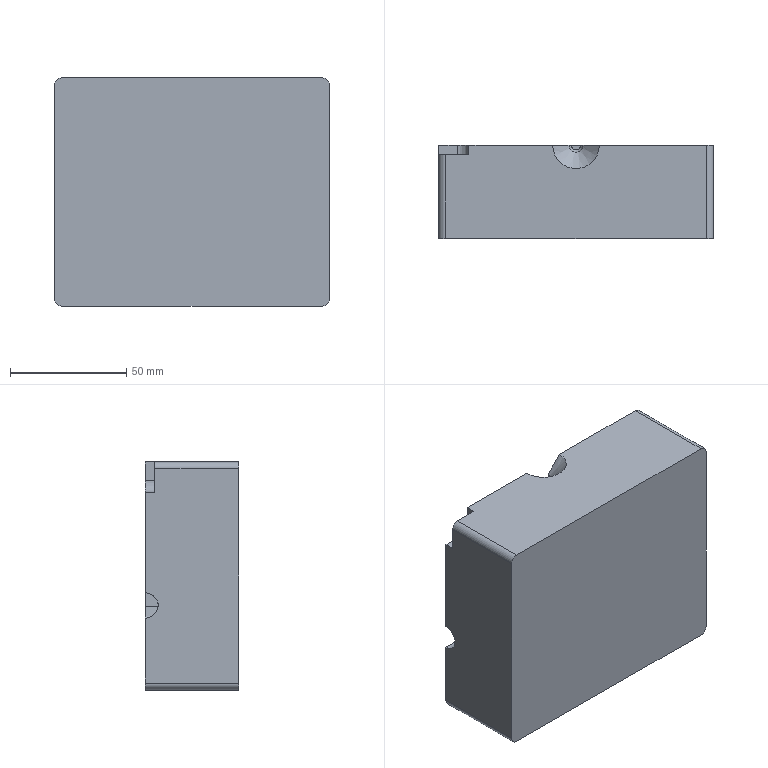NC program | NX | posted with a generic post | part box 118 x 40 x 98 mm
Lines 34771 to 36173 of 39656:
(ZLEVEL_PROFILE , TOOL : D8R1)
N69516 M6
N69518 G54
N69520 G17 G0 G90 X14.157 Y-3.614 S0 M3
N69522 G43 Z30. H0
N69524 Z3.
N69526 G94 G1 Z-5. F250.
N69528 G2 X13.635 Y-1.241 R6.575
N69530 G1 X13.195 Y13.066
N69532 G3 X-13.195 Y13.066 R13.201
N69534 G1 X-13.635 Y-1.241
N69536 G2 X-14.157 Y-3.614 R6.575
N69538 G1 Z-8.446
N69540 G3 X-13.635 Y-1.241 R6.575
N69542 G1 X-13.195 Y13.066
N69544 G2 X13.195 Y13.066 R13.201
N69546 G1 X13.635 Y-1.241
N69548 G3 X14.157 Y-3.614 R6.575
N69550 G1 Z-8.546
N69552 G2 X13.747 Y-2.265 R6.575
N69554 X13.637 Y-1.375 R4.842
N69556 G1 X13.192 Y13.066
N69558 G3 X-13.192 Y13.066 R13.199
N69560 G1 X-13.62 Y-0.843
N69562 X-13.625 Y-1.126
N69564 G2 X-14.153 Y-3.614 R6.711
N69566 G1 X-14.144 Z-8.646
N69568 G3 X-13.625 Y-1.241 R6.517
N69570 G1 X-13.185 Y13.066
N69572 G2 X13.185 Y13.066 R13.191
N69574 G1 X13.63 Y-1.399
N69576 G3 X13.773 Y-2.439 R4.96
N69578 X13.926 Y-3.018 R3.566
N69580 X14.145 Y-3.614 R6.362
N69582 G1 X14.132 Z-8.745
N69584 G2 X13.684 Y-2.04 R6.455
N69586 G1 X13.629 Y-1.641
N69588 X13.624 Y-1.58
N69590 X13.173 Y13.065
N69592 G3 X-13.173 Y13.065 R13.179
N69594 G1 X-13.613 Y-1.24
N69596 G2 X-14.133 Y-3.614 R6.519
N69598 G1 X-14.119 Z-8.843
N69600 G3 X-13.596 Y-1.24 R6.527
N69602 G1 X-13.156 Y13.065
N69604 G2 X13.156 Y13.065 R13.162
N69606 G1 X13.601 Y-1.412
N69608 X13.602 Y-1.426
N69610 G3 X14.118 Y-3.614 R6.556
N69612 G1 X14.101 Z-8.941
N69614 G2 X13.571 Y-1.239 R6.593
N69616 G1 X13.562 Y-0.843
N69618 X13.134 Y13.064
N69620 G3 X-13.134 Y13.064 R13.141
N69622 G1 X-13.575 Y-1.241
N69624 G2 X-14.1 Y-3.614 R6.53
N69626 G1 X-14.074 Z-9.037
N69628 G3 X-13.548 Y-1.242 R6.515
N69630 G1 X-13.108 Y13.063
N69632 G2 X13.108 Y13.063 R13.114
N69634 G1 X13.548 Y-1.242
N69636 G3 X14.075 Y-3.614 R6.53
N69638 G1 X14.036 Z-9.13
N69640 G2 X13.518 Y-1.242 R6.424
N69642 G1 X13.078 Y13.062
N69644 G3 X-13.078 Y13.062 R13.084
N69646 G1 X-13.519 Y-1.274
N69648 G2 X-14.036 Y-3.614 R6.424
N69650 G1 X-13.99 Z-9.221
N69652 G3 X-13.484 Y-1.242 R6.349
N69654 G1 X-13.044 Y13.061
N69656 G2 X13.044 Y13.061 R13.05
N69658 G1 X13.485 Y-1.305
N69660 G3 X13.988 Y-3.614 R6.337
N69662 G1 X13.935 Z-9.308
N69664 G2 X13.449 Y-1.345 R6.247
N69666 G1 X13.006 Y13.06
N69668 G3 X-13.006 Y13.06 R13.012
N69670 G1 X-13.449 Y-1.345
N69672 G2 X-13.934 Y-3.614 R6.251
N69674 G1 X-13.877 Z-9.392
N69676 G3 X-13.409 Y-1.392 R6.194
N69678 G1 X-12.965 Y13.059
N69680 G2 X12.965 Y13.059 R12.971
N69682 G1 X13.409 Y-1.392
N69684 G3 X13.875 Y-3.614 R6.153
N69686 G1 X13.808 Z-9.474
N69688 G2 X13.366 Y-1.448 R6.078
N69690 G1 X12.92 Y13.057
N69692 G3 X-12.92 Y13.057 R12.926
N69694 G1 X-13.366 Y-1.448
N69696 G2 X-13.813 Y-3.614 R6.117
N69698 G1 Z-6.474
N69700 G0 Z30.
N69702 X-13.744
N69704 Z-6.474
N69706 G1 Z-9.552
N69708 G3 X-13.323 Y-1.571 R6.07
N69710 G1 X-12.873 Y13.056
N69712 G2 X12.873 Y13.056 R12.879
N69714 G1 X13.321 Y-1.508
N69716 G3 X13.743 Y-3.614 R6.057
N69718 G1 X13.67 Z-9.627
N69720 G2 X13.273 Y-1.576 R5.974
N69722 G1 X12.823 Y13.054
N69724 G3 X-12.823 Y13.054 R12.829
N69726 G1 X-13.274 Y-1.637
N69728 G2 X-13.672 Y-3.614 R6.048
N69730 G1 X-13.593 Z-9.7
N69732 G3 X-13.468 Y-3.238 R5.87
N69734 X-13.224 Y-1.718 R6.009
N69736 G1 X-12.77 Y13.053
N69738 G2 X12.77 Y13.053 R12.776
N69740 G1 X13.222 Y-1.641
N69742 G3 X13.593 Y-3.614 R5.887
N69744 G1 X13.516 Z-9.768
N69746 G2 X13.172 Y-1.814 R5.817
N69748 G1 X12.715 Y13.051
N69750 G3 X-12.715 Y13.051 R12.721
N69752 G1 X-13.169 Y-1.724
N69754 G2 X-13.515 Y-3.614 R5.802
N69756 G1 X-13.433 Z-9.835
N69758 G3 X-13.113 Y-1.806 R5.719
N69760 G1 X-12.657 Y13.049
N69762 G2 X12.657 Y13.049 R12.663
N69764 G1 X13.113 Y-1.805
N69766 G3 X13.435 Y-3.614 R5.767
N69768 G1 X13.351 Z-9.899
N69770 G2 X13.055 Y-1.89 R5.702
N69772 G1 X12.596 Y13.047
N69774 G3 X-12.596 Y13.047 R12.602
N69776 G1 X-13.055 Y-1.89
N69778 G2 X-13.35 Y-3.614 R5.666
N69780 G1 X-13.263 Z-9.96
N69782 G3 X-12.995 Y-1.978 R5.581
N69784 G1 X-12.532 Y13.046
N69786 G2 X12.532 Y13.046 R12.538
N69788 G1 X12.995 Y-1.978
N69790 G3 X13.263 Y-3.614 R5.586
N69792 G1 X13.176 Z-10.018
N69794 G2 X12.944 Y-2.257 R5.429
N69796 G1 X12.919 Y-1.641
N69798 X12.467 Y13.043
N69800 G3 X-12.467 Y13.044 R12.473
N69802 G1 X-12.932 Y-2.068
N69804 G2 X-13.175 Y-3.614 R5.478
N69806 G1 X-13.086 Z-10.072
N69808 G3 X-12.871 Y-2.264 R5.365
N69810 G1 X-12.4 Y13.041
N69812 G2 X12.4 Y13.041 R12.406
N69814 G1 X12.867 Y-2.159
N69816 G3 X13.087 Y-3.614 R5.432
N69818 G1 X12.997 Z-10.125
N69820 G2 X12.799 Y-2.253 R5.355
N69822 G1 X12.329 Y13.039
N69824 G3 X-12.329 Y13.039 R12.335
N69826 G1 X-12.799 Y-2.253
N69828 G2 X-12.996 Y-3.614 R5.31
N69830 G1 X-12.905 Z-10.175
N69832 G3 X-12.731 Y-2.425 R5.255
N69834 G1 X-12.256 Y13.037
N69836 G2 X12.256 Y13.037 R12.261
N69838 G1 X12.732 Y-2.434
N69840 G3 X12.904 Y-3.614 R5.237
N69842 G1 X12.862 Z-10.198
N69844 X12.814 Z-10.221
N69846 G2 X12.67 Y-2.618 R5.14
N69848 G1 X12.644 Y-2.04
N69850 X12.18 Y13.035
N69852 G3 X-12.18 Y13.035 R12.186
N69854 G1 X-12.657 Y-2.49
N69856 G2 X-12.815 Y-3.614 R5.237
N69858 G1 X-12.768 Z-10.243
N69860 X-12.721 Z-10.264
N69862 G3 X-12.582 Y-2.534 R5.115
N69864 G1 X-12.103 Y13.032
N69866 G2 X12.103 Y13.032 R12.109
N69868 G1 X12.582 Y-2.534
N69870 G3 X12.717 Y-3.614 R5.084
N69872 G1 X12.673 Z-10.285
N69874 X12.62 Z-10.305
N69876 G2 X12.505 Y-2.625 R4.917
N69878 G1 X12.023 Y13.03
N69880 G3 X-12.023 Y13.03 R12.029
N69882 G1 X-12.505 Y-2.625
N69884 G2 X-12.624 Y-3.614 R4.949
N69886 G1 X-12.58 Z-10.323
N69888 X-12.529 Z-10.342
N69890 G3 X-12.425 Y-2.712 R4.887
N69892 G1 X-11.941 Y13.027
N69894 G2 X11.941 Y13.027 R11.947
N69896 G1 X12.425 Y-2.712
N69898 G3 X12.525 Y-3.614 R4.837
N69900 G1 X12.484 Z-10.359
N69902 X12.428 Z-10.375
N69904 G2 X12.344 Y-2.794 R4.705
N69906 G1 X11.857 Y13.025
N69908 G3 X-11.857 Y13.025 R11.863
N69910 G1 X-12.344 Y-2.793
N69912 G2 X-12.431 Y-3.614 R4.768
N69914 G1 X-12.387 Z-10.39
N69916 X-12.334 Z-10.405
N69918 G3 X-12.261 Y-2.867 R4.637
N69920 G1 X-11.772 Y13.022
N69922 G2 X11.772 Y13.022 R11.778
N69924 G1 X12.261 Y-2.867
N69926 G3 X12.333 Y-3.614 R4.595
N69928 G1 X12.298 Z-10.418
N69930 X12.242 Z-10.431
N69932 G2 X12.176 Y-2.932 R4.607
N69934 G1 X11.685 Y13.019
N69936 G3 X-11.685 Y13.019 R11.691
N69938 G1 X-12.176 Y-2.932
N69940 G2 X-12.239 Y-3.614 R4.517
N69942 G1 X-12.2 Z-10.442
N69944 X-12.145 Z-10.453
N69946 G3 X-12.091 Y-2.986 R4.38
N69948 G1 X-11.598 Y13.017
N69950 G2 X11.598 Y13.017 R11.604
N69952 G1 X12.091 Y-2.986
N69954 G3 X12.15 Y-3.614 R4.595
N69956 G1 X12.114 Z-10.462
N69958 X12.061 Z-10.471
N69960 G2 X12.006 Y-3.026 R4.52
N69962 G1 X11.513 Y13.014
N69964 G3 X-11.513 Y13.014 R11.518
N69966 G1 X-12.006 Y-3.026
N69968 G2 X-12.057 Y-3.614 R4.367
N69970 G1 X-12.023 Z-10.478
N69972 X-11.974 Z-10.485
N69974 G3 X-11.923 Y-3.042 R4.396
N69976 G1 X-11.429 Y13.012
N69978 G2 X11.429 Y13.012 R11.434
N69980 G1 X11.923 Y-3.066
N69982 G3 X11.975 Y-3.614 R4.404
N69984 G1 X11.943 Z-10.489
N69986 X11.907 Z-10.494
N69988 G2 X11.855 Y-3.067 R4.356
N69990 G1 X11.361 Y13.009
N69992 G3 X-11.361 Y13.009 R11.366
N69994 G1 X-11.855 Y-3.067
N69996 G2 X-11.909 Y-3.614 R4.432
N69998 G1 Z-7.494
N70000 G0 Z30.
N70002 X-11.725 Y-2.838
N70004 Z-7.494
N70006 G1 Z-10.506
N70008 X-11.237 Y13.006
N70010 G2 X11.237 Y13.006 R11.242
N70012 G1 X11.709 Y-2.323
N70014 Z-10.504
N70016 X11.607 Y-2.326 Z-10.506
N70018 X8.71 Y-2.415
N70020 X8.346 Y-2.398
N70022 X7.154 Y-2.352
N70024 X5.564 Y-2.305
N70026 X4.372 Y-2.277
N70028 X2.782 Y-2.251
N70030 X1.987 Y-2.244
N70032 X1.192 Y-2.238
N70034 X-0.397 Y-2.235
N70036 X-1.59 Y-2.24
N70038 X-3.179 Y-2.256
N70040 X-4.769 Y-2.285
N70042 X-6.359 Y-2.327
N70044 X-7.551 Y-2.367
N70046 X-8.71 Y-2.414
N70048 X-8.239 Y12.913
N70050 G2 X8.239 Y12.913 R8.242
N70052 G1 X8.71 Y-2.415
N70054 X5.613 Y0.695
N70056 X4.443 Y0.723
N70058 X4.42
N70060 X-1.621 Y0.76
N70062 X-5.613 Y0.694
N70064 X-5.24 Y12.821
N70066 G2 X5.24 Y12.821 R5.242
N70068 G1 X5.613 Y0.695
N70070 X2.518 Y3.735
N70072 X-1.627 Y3.76
N70074 X-2.518 Y3.751
N70076 X-2.241 Y12.729
N70078 G2 X2.241 Y12.729 R2.242
N70080 G1 X2.518 Y3.735
N70082 X11.605 Y-2.254
N70084 X11.709 Y-2.323 Z-10.504
N70086 Z-10.506
N70088 X11.723 Y-2.791
N70090 Z-7.506
N70092 G0 Z30.
N70094 M5
(CONTOUR_AREA_COPY_COPY , TOOL : B4)
N70096 M6
N70098 G54
N70100 G17 G0 G90 X1.987 Y-7.133 S0 M3
N70102 G43 Z30. H0
N70104 Z1.2
N70106 G94 G1 Z-11.524 F250.
N70108 G3 X-0.002 Y-5.122 R2.
N70110 G1 X-0.397 Y-5.12 Z-11.523
N70112 X-1.588 Y-5.123 Z-11.519
N70114 X-1.985 Y-5.122 Z-11.516
N70116 X-2.78 Y-5.117 Z-11.507
N70118 X-3.177 Y-5.119 Z-11.503
N70120 X-3.971 Z-11.491
N70122 X-5.162 Y-5.112 Z-11.468
N70124 X-5.956 Z-11.45
N70126 X-6.75 Y-5.109 Z-11.428
N70128 X-7.544 Y-5.101 Z-11.404
N70130 X-7.942 Z-11.392
N70132 X-8.736 Y-5.099 Z-11.364
N70134 X-9.927 Y-5.088 Z-11.317
N70136 X-10.324 Y-5.084 Z-11.3
N70138 X-11.118 Y-5.082 Z-11.263
N70140 X-11.913 Y-5.081 Z-11.228
N70142 X-12.211 Y-5.09 Z-11.22
N70144 X-12.31 Y-5.093 Z-11.214
N70146 X-13.104 Y-5.116 Z-11.172
N70148 X-14.693 Y-5.17 Z-11.078
N70150 X-15.09 Y-5.186 Z-11.054
N70152 X-15.486 Y-5.199 Z-11.028
N70154 X-15.883 Z-11.002
N70156 X-16.279 Y-5.179 Z-10.974
N70158 X-16.676 Y-5.141 Z-10.947
N70160 X-17.073 Y-5.087 Z-10.915
N70162 X-17.175 Y-5.085 Z-10.9
N70164 X-17.74 Y-5.132 Z-10.856
N70166 X-18.066 Y-5.167 Z-10.828
N70168 X-18.259 Y-5.193 Z-10.811
N70170 X-18.128 Y-5.131 Z-10.77
N70172 X-18.007 Y-5.067 Z-10.729
N70174 X-17.894 Y-5.002 Z-10.693
N70176 X-17.861 Y-4.984 Z-10.682
N70178 X-17.685 Y-4.873 Z-10.626
N70180 X-17.463 Y-4.718 Z-10.561
N70182 X-17.317 Y-4.605 Z-10.523
N70184 X-17.176 Y-4.485 Z-10.487
N70186 X-17.064 Y-4.384 Z-10.459
N70188 X-16.784 Y-4.098 Z-10.399
N70190 X-16.666 Y-3.96 Z-10.377
N70192 X-16.568 Y-3.837 Z-10.363
N70194 X-16.473 Y-3.71 Z-10.351
N70196 X-16.268 Y-3.395 Z-10.333
N70198 X-16.225 Y-3.323 Z-10.331
N70200 X-16.026 Y-2.935 Z-10.338
N70202 X-15.871 Y-2.548 Z-10.363
N70204 X-15.829 Y-2.419 Z-10.372
N70206 X-15.79 Y-2.289 Z-10.384
N70208 X-15.755 Y-2.16 Z-10.399
N70210 X-15.736 Y-2.083 Z-10.405
N70212 X-15.704 Y-1.928 Z-10.42
N70214 X-15.675 Y-1.773 Z-10.44
N70216 X-15.648 Y-1.596 Z-10.464
N70218 X-15.65 Y-1.674 Z-10.466
N70220 X-15.653 Y-2.097 Z-10.481
N70222 X-15.656 Y-2.52 Z-10.492
N70224 Y-2.81 Z-10.499
N70226 X-15.653 Y-2.931 Z-10.502
N70228 X-15.649 Y-2.958 Z-10.503
N70230 X-15.627 Y-2.962 Z-10.506
N70232 X-15.617 Y-2.943
N70234 X-15.583 Y-2.937
N70236 G2 X-6.502 Y-2.361 R123.1
N70238 G1 X-4.666 Y-2.312
N70240 G2 X8.736 Y-2.441 R210.057
N70242 G1 X11.117 Y-2.567
N70244 X13.303 Y-2.722
N70246 X15.615 Y-2.939
N70248 X15.625 Y-2.966
N70250 X15.648 Y-2.964 Z-10.504
N70252 X15.653 Y-2.931 Z-10.502
N70254 X15.656 Y-2.87 Z-10.5
N70256 X15.655 Y-2.285 Z-10.487
N70258 X15.652 Y-1.847 Z-10.473
N70260 X15.65 Y-1.77 Z-10.471
N70262 Y-1.654 Z-10.464
N70264 X15.649 Y-1.615 Z-10.463
N70266 X15.648 Y-1.576 Z-10.461
N70268 X15.668 Y-1.734 Z-10.448
N70270 X15.675 Y-1.773 Z-10.444
N70272 X15.689 Y-1.85 Z-10.435
N70274 X15.72 Y-2.005 Z-10.418
N70276 X15.755 Y-2.16 Z-10.398
N70278 X15.79 Y-2.289 Z-10.385
N70280 X15.829 Y-2.419 Z-10.372
N70282 X15.869 Y-2.54 Z-10.362
N70284 X16.026 Y-2.935 Z-10.337
N70286 X16.225 Y-3.323 Z-10.33
N70288 X16.268 Y-3.395 Z-10.332
N70290 X16.473 Y-3.71 Z-10.352
N70292 X16.666 Y-3.96 Z-10.379
N70294 X16.784 Y-4.098 Z-10.402
N70296 X17.064 Y-4.387 Z-10.464
N70298 X17.12 Y-4.437 Z-10.475
N70300 X17.176 Y-4.486 Z-10.487
N70302 X17.463 Y-4.719 Z-10.565
N70304 X17.685 Y-4.873 Z-10.631
N70306 X17.861 Y-4.982 Z-10.681
N70308 X18.007 Y-5.067 Z-10.731
N70310 X18.129 Y-5.131 Z-10.77
N70312 X18.256 Y-5.192 Z-10.81
N70314 X18.069 Y-5.166 Z-10.827
N70316 X17.87 Y-5.145 Z-10.844
N70318 X17.738 Y-5.128 Z-10.855
N70320 X17.605 Y-5.118 Z-10.866
N70322 X17.274 Y-5.088 Z-10.892
N70324 X17.174 Y-5.085 Z-10.9
N70326 X17.073 Y-5.087 Z-10.915
N70328 X17.072
N70330 X16.414 Y-5.164 Z-10.965
N70332 X15.752 Y-5.198 Z-11.01
N70334 X15.09 Y-5.186 Z-11.054
N70336 X13.898 Y-5.141 Z-11.127
N70338 X12.055 Y-5.086 Z-11.228
N70340 X11.913 Y-5.082 Z-11.232
N70342 X11.515 Y-5.077 Z-11.245
N70344 X10.721 Y-5.08 Z-11.282
N70346 X9.927 Y-5.089 Z-11.317
N70348 X8.736 Y-5.093 Z-11.363
N70350 X8.339 Y-5.099 Z-11.378
N70352 X7.942 Y-5.102 Z-11.392
N70354 X6.75 Y-5.106 Z-11.428
N70356 X5.956 Y-5.111 Z-11.45
N70358 X4.765 Y-5.114 Z-11.476
N70360 X3.971 Y-5.118 Z-11.491
N70362 X3.177 Y-5.12 Z-11.503
N70364 X2.382 Y-5.119 Z-11.511
N70366 X1.588 Y-5.122 Z-11.519
N70368 X0. Z-11.524
N70370 X-0.002
N70372 X-0.001 Y-5.022 Z-11.446
N70374 X-0.397 Y-5.02 Z-11.445
N70376 X-1.588 Y-5.023 Z-11.441
N70378 X-1.985 Y-5.022 Z-11.438
N70380 X-2.779 Y-5.017 Z-11.43
N70382 X-3.177 Y-5.019 Z-11.426
N70384 X-3.97 Z-11.415
N70386 X-5.162 Y-5.012 Z-11.393
N70388 X-5.956 Z-11.375
N70390 X-6.75 Y-5.009 Z-11.355
N70392 X-7.544 Y-5.001 Z-11.333
N70394 X-7.941 Z-11.321
N70396 X-8.735 Y-4.999 Z-11.294
N70398 X-9.926 Y-4.988 Z-11.251
N70400 X-10.323 Y-4.984 Z-11.235
N70402 X-11.118 Y-4.982 Z-11.199
N70404 X-11.914 Y-4.981 Z-11.164
N70406 X-12.313 Y-4.993 Z-11.155
N70408 X-13.107 Y-5.016 Z-11.137
N70410 X-14.498 Y-5.063 Z-11.09
N70412 X-14.696 Y-5.07 Z-11.078
N70414 X-15.093 Y-5.087 Z-11.054
N70416 X-15.488 Y-5.099 Z-11.028
N70418 X-15.88 Z-11.002
N70420 X-16.272 Y-5.079 Z-10.975
N70422 X-16.529 Y-5.054 Z-10.957
N70424 X-16.664 Y-5.041 Z-10.935
N70426 X-17.066 Y-4.987 Z-10.848
N70428 X-17.178 Y-4.985 Z-10.83
N70430 X-17.748 Y-5.032 Z-10.761
N70432 X-17.75 Z-10.76
N70434 X-17.63 Y-4.956 Z-10.72
N70436 X-17.404 Y-4.798 Z-10.645
N70438 X-17.254 Y-4.683 Z-10.6
N70440 X-17.11 Y-4.561 Z-10.558
N70442 X-16.995 Y-4.456 Z-10.53
N70444 X-16.711 Y-4.166 Z-10.462
N70446 X-16.589 Y-4.024 Z-10.44
N70448 X-16.489 Y-3.898 Z-10.423
N70450 X-16.391 Y-3.768 Z-10.407
N70452 X-16.182 Y-3.448 Z-10.39
N70454 X-16.138 Y-3.371 Z-10.387
N70456 X-15.935 Y-2.977 Z-10.398
N70458 X-15.934 Y-2.974
N70460 X-15.777 Y-2.582 Z-10.43
N70462 X-15.756 Y-2.52 Z-10.435
N70464 Y-2.812 Z-10.46
N70466 X-15.753 Y-2.94 Z-10.471
N70468 X-15.747 Y-2.974 Z-10.476
N70470 X-15.719 Y-3.029 Z-10.488
N70472 X-15.664 Y-3.057 Z-10.503
N70474 X-15.643 Y-3.061 Z-10.507
N70476 X-15.598 Y-3.057 Z-10.509
N70478 X-15.559 Y-3.035
N70480 X-14.357 Y-2.92 Z-10.508
N70482 X-13.154 Y-2.816
N70484 X-11.95 Y-2.726 Z-10.509
N70486 X-10.746 Y-2.647 Z-10.508
N70488 X-9.54 Y-2.58
N70490 G2 X8.731 Y-2.541 R209.383
N70492 G1 X11.111 Y-2.667
N70494 X13.295 Y-2.822
N70496 X15.475 Y-3.027 Z-10.509
N70498 X15.551 Y-3.034
N70500 X15.59 Y-3.06
N70502 X15.636 Y-3.066 Z-10.507
N70504 X15.659 Y-3.063 Z-10.505
N70506 X15.718 Y-3.036 Z-10.49
N70508 X15.747 Y-2.978 Z-10.476
N70510 X15.753 Y-2.941 Z-10.471
N70512 X15.756 Y-2.873 Z-10.465
N70514 Y-2.572 Z-10.441
N70516 Y-2.517 Z-10.435
N70518 X15.775 Y-2.574 Z-10.429
N70520 X15.935 Y-2.977 Z-10.397
N70522 X16.138 Y-3.371 Z-10.387
N70524 X16.182 Y-3.448 Z-10.388
N70526 X16.392 Y-3.768 Z-10.407
N70528 X16.588 Y-4.023 Z-10.439
N70530 X16.71 Y-4.165 Z-10.462
N70532 X16.995 Y-4.46 Z-10.532
N70534 X17.054 Y-4.512 Z-10.548
N70536 X17.111 Y-4.562 Z-10.564
N70538 X17.402 Y-4.799 Z-10.651
N70540 X17.63 Y-4.957 Z-10.721
N70542 X17.746 Y-5.028 Z-10.761
N70544 X17.613 Y-5.018 Z-10.779
N70546 X17.28 Y-4.988 Z-10.816
N70548 X17.175 Y-4.985 Z-10.83
N70550 X17.065 Y-4.987 Z-10.849
N70552 X16.738 Y-5.031 Z-10.917
N70554 X16.483 Y-5.058 Z-10.96
N70556 X16.411 Y-5.064 Z-10.965
N70558 X15.753 Y-5.098 Z-11.01
N70560 X15.095 Y-5.087 Z-11.053
N70562 X14.2 Y-5.059 Z-11.108
N70564 X13.305 Y-5.032 Z-11.137
N70566 X11.516 Y-4.977 Z-11.182
N70568 X10.72 Y-4.98 Z-11.219
N70570 X9.926 Y-4.989 Z-11.25
N70572 X8.735 Y-4.993 Z-11.295
N70574 X8.337 Y-4.999 Z-11.309
N70576 X7.941 Y-5.002 Z-11.321
N70578 X6.75 Y-5.006 Z-11.356
N70580 X5.956 Y-5.011 Z-11.376
N70582 X4.765 Y-5.014 Z-11.401
N70584 X3.97 Y-5.018 Z-11.415
N70586 X3.177 Y-5.02 Z-11.425
N70588 X2.382 Y-5.019 Z-11.434
N70590 X1.588 Y-5.022 Z-11.441
N70592 X0. Z-11.446
N70594 X-0.001
N70596 Y-4.972 Z-11.407
N70598 Y-4.922 Z-11.371
N70600 X-0.397 Y-4.92 Z-11.369
N70602 X-1.588 Y-4.923 Z-11.366
N70604 X-1.985 Y-4.922 Z-11.363
N70606 X-2.779 Y-4.917 Z-11.356
N70608 X-3.177 Y-4.919 Z-11.352
N70610 X-3.97 Z-11.341
N70612 X-5.161 Y-4.912 Z-11.321
N70614 X-5.956 Z-11.305
N70616 X-6.749 Y-4.909 Z-11.286
N70618 X-7.543 Y-4.901 Z-11.264
N70620 X-7.941 Z-11.253
N70622 X-8.735 Y-4.899 Z-11.228
N70624 X-9.925 Y-4.888 Z-11.187
N70626 X-10.323 Y-4.884 Z-11.171
N70628 X-11.118 Y-4.882 Z-11.138
N70630 X-11.916 Y-4.881 Z-11.107
N70632 X-12.316 Y-4.893 Z-11.099
N70634 X-13.11 Y-4.916 Z-11.081
N70636 X-14.7 Y-4.97 Z-11.032
N70638 X-15.097 Y-4.987 Z-11.022
N70640 X-15.489 Y-4.999 Z-11.006
N70642 X-15.878 Z-10.978
N70644 X-16.265 Y-4.979 Z-10.936
N70646 X-16.653 Y-4.942 Z-10.878
N70648 X-17.058 Y-4.887 Z-10.783
N70650 X-17.181 Y-4.885 Z-10.76
N70652 X-17.376 Y-4.901 Z-10.733
N70654 X-17.344 Y-4.879 Z-10.724
N70656 X-17.191 Y-4.761 Z-10.672
N70658 X-17.044 Y-4.636 Z-10.626
N70660 X-16.925 Y-4.528 Z-10.595
N70662 X-16.637 Y-4.233 Z-10.52
N70664 X-16.512 Y-4.088 Z-10.495
N70666 X-16.409 Y-3.959 Z-10.472
N70668 X-16.309 Y-3.825 Z-10.459
N70670 X-16.097 Y-3.5 Z-10.436
N70672 X-16.05 Y-3.419 Z-10.435
N70674 X-15.841 Y-3.012 Z-10.444
N70676 X-15.782 Y-3.108 Z-10.476
N70678 X-15.68 Y-3.156 Z-10.505
N70680 X-15.598 Y-3.16 Z-10.512
N70682 X-15.521 Y-3.131
N70684 X-14.325 Y-3.017
N70686 X-13.128 Y-2.915
N70688 X-11.929 Y-2.824 Z-10.513
N70690 X-10.73 Y-2.746 Z-10.511
N70692 X-9.531 Y-2.679
N70694 X-8.33 Y-2.625 Z-10.513
N70696 X-6.496 Y-2.561 Z-10.512
N70698 X-4.662 Y-2.512 Z-10.511
N70700 X-2.827 Y-2.48
N70702 X-0.992 Y-2.463 Z-10.512
N70704 X0.843 Y-2.462
N70706 X2.678 Y-2.477 Z-10.511
N70708 X4.513 Y-2.508
N70710 X6.347 Y-2.554
N70712 X8.727 Y-2.641 Z-10.512
N70714 X11.105 Y-2.767 Z-10.513
N70716 X13.287 Y-2.922 Z-10.511
N70718 X15.465 Y-3.126 Z-10.512
N70720 X15.511 Y-3.131
N70722 X15.576 Y-3.16 Z-10.513
N70724 X15.647 Y-3.165 Z-10.51
N70726 X15.711 Y-3.155 Z-10.499
N70728 X15.768 Y-3.125 Z-10.481
N70730 X15.815 Y-3.076 Z-10.462
N70732 X15.842 Y-3.013 Z-10.445
N70734 X15.946 Y-3.216 Z-10.432
N70736 X16.05 Y-3.419 Z-10.435
N70738 X16.097 Y-3.5 Z-10.437
N70740 X16.31 Y-3.826 Z-10.458
N70742 X16.511 Y-4.086 Z-10.494
N70744 X16.636 Y-4.233 Z-10.518
N70746 X16.926 Y-4.532 Z-10.593
N70748 X16.988 Y-4.587 Z-10.61
N70750 X17.047 Y-4.638 Z-10.629
N70752 X17.342 Y-4.879 Z-10.726
N70754 X17.366 Y-4.895 Z-10.733
N70756 X17.287 Y-4.888 Z-10.742
N70758 X17.175 Y-4.885 Z-10.761
N70760 X17.056 Y-4.887 Z-10.786
N70762 X16.406 Y-4.964 Z-10.917
N70764 X15.753 Y-4.998 Z-10.986
N70766 X15.099 Y-4.987 Z-11.019
N70768 X13.308 Y-4.932 Z-11.079
N70770 X11.517 Y-4.877 Z-11.123
N70772 X10.719 Y-4.88 Z-11.156
N70774 X9.925 Y-4.889 Z-11.187
N70776 X8.734 Y-4.893 Z-11.227
N70778 X8.336 Y-4.899 Z-11.241
N70780 X7.94 Y-4.902 Z-11.253
N70782 X6.749 Y-4.906 Z-11.286
N70784 X5.955 Y-4.911 Z-11.305
N70786 X4.764 Y-4.914 Z-11.328
N70788 X3.97 Y-4.918 Z-11.341
N70790 X3.177 Y-4.92 Z-11.352
N70792 X2.382 Y-4.919 Z-11.359
N70794 X1.588 Y-4.922 Z-11.366
N70796 X0.001 Z-11.371
N70798 X-0.001
N70800 X0. Y-4.822 Z-11.302
N70802 X-0.397 Y-4.82 Z-11.301
N70804 X-1.588 Y-4.823 Z-11.297
N70806 X-1.984 Y-4.822 Z-11.295
N70808 X-2.779 Y-4.817 Z-11.288
N70810 X-3.177 Y-4.819 Z-11.284
N70812 X-3.97 Z-11.274
N70814 X-5.161 Y-4.812 Z-11.255
N70816 X-5.956 Z-11.239
N70818 X-6.748 Y-4.809 Z-11.22
N70820 X-7.543 Y-4.801 Z-11.201
N70822 X-7.941 Z-11.191
N70824 X-8.734 Y-4.799 Z-11.166
N70826 X-9.924 Y-4.788 Z-11.128
N70828 X-10.322 Y-4.784 Z-11.113
N70830 X-11.118 Y-4.782 Z-11.082
N70832 X-11.917 Y-4.781 Z-11.051
N70834 X-12.319 Y-4.793 Z-11.043
N70836 X-13.114 Y-4.816 Z-11.026
N70838 X-14.704 Y-4.87 Z-10.981
N70840 X-15.1 Y-4.887 Z-10.971
N70842 X-15.491 Y-4.899 Z-10.956
N70844 X-15.875 Z-10.932
N70846 X-16.257 Y-4.88 Z-10.885
N70848 X-16.641 Y-4.843 Z-10.824
N70850 X-17.051 Y-4.787 Z-10.721
N70852 X-17.067 Z-10.717
N70854 X-16.978 Y-4.711 Z-10.689
N70856 X-16.856 Y-4.6 Z-10.653
N70858 X-16.563 Y-4.301 Z-10.572
N70860 X-16.435 Y-4.151 Z-10.541
N70862 X-16.33 Y-4.02 Z-10.518
N70864 X-16.227 Y-3.882 Z-10.503
N70866 X-16.012 Y-3.553 Z-10.477
N70868 X-15.962 Y-3.466 Z-10.476
N70870 X-15.825 Y-3.201 Z-10.472
N70872 X-15.766 Y-3.234 Z-10.493
N70874 X-15.701 Y-3.254 Z-10.509
N70876 X-15.593 Y-3.261 Z-10.519
N70878 X-15.49 Y-3.229 Z-10.517
N70880 X-14.298 Y-3.115 Z-10.518
N70882 X-13.105 Y-3.013
N70884 X-10.717 Y-2.845
N70886 X-8.326 Y-2.725 Z-10.517
N70888 X-6.493 Y-2.661
N70890 X-4.66 Y-2.612 Z-10.518
N70892 X-2.826 Y-2.58 Z-10.516
N70894 X-0.992 Y-2.563 Z-10.517
N70896 X0.842 Y-2.562 Z-10.516
N70898 X2.677 Y-2.577
N70900 X4.51 Y-2.608 Z-10.518
N70902 X6.344 Y-2.654 Z-10.517
N70904 X8.722 Y-2.741
N70906 X11.099 Y-2.866 Z-10.518
N70908 X13.279 Y-3.021
N70910 X15.455 Y-3.226 Z-10.517
N70912 X15.478 Y-3.228
N70914 X15.563 Y-3.26 Z-10.519
N70916 X15.652 Y-3.265 Z-10.515
N70918 X15.745 Y-3.249 Z-10.499
N70920 X15.828 Y-3.205 Z-10.474
N70922 X15.962 Y-3.466 Z-10.473
N70924 X16.012 Y-3.553 Z-10.477
N70926 X16.229 Y-3.884 Z-10.502
N70928 X16.433 Y-4.149 Z-10.54
N70930 X16.562 Y-4.3 Z-10.57
N70932 X16.857 Y-4.604 Z-10.653
N70934 X16.982 Y-4.715 Z-10.69
N70936 X17.071 Y-4.787 Z-10.718
N70938 X17.047 Z-10.723
N70940 X16.725 Y-4.831 Z-10.804
N70942 X16.402 Y-4.864 Z-10.863
N70944 X15.753 Y-4.898 Z-10.939
N70946 X15.103 Y-4.887 Z-10.969
N70948 X13.311 Y-4.832 Z-11.026
N70950 X11.519 Y-4.777 Z-11.067
N70952 X10.719 Y-4.78 Z-11.099
N70954 X9.925 Y-4.789 Z-11.127
N70956 X8.733 Y-4.793 Z-11.167
N70958 X8.335 Y-4.799 Z-11.179
N70960 X7.94 Y-4.802 Z-11.19
N70962 X6.749 Y-4.806 Z-11.222
N70964 X5.955 Y-4.811 Z-11.239
N70966 X4.764 Y-4.814 Z-11.262
N70968 X3.969 Y-4.818 Z-11.274
N70970 X3.177 Y-4.82 Z-11.283
N70972 X2.382 Y-4.819 Z-11.291
N70974 X1.588 Y-4.822 Z-11.297
N70976 X0.001 Z-11.302
N70978 X0. Y-4.722 Z-11.234
N70980 X-0.396 Y-4.72 Z-11.233
N70982 X-1.589 Y-4.723 Z-11.23
N70984 X-1.984 Y-4.722 Z-11.228
N70986 X-2.779 Y-4.717 Z-11.221
N70988 X-3.178 Y-4.719 Z-11.217
N70990 X-3.97 Z-11.208
N70992 X-5.161 Y-4.712 Z-11.19
N70994 X-5.955 Z-11.176
N70996 X-6.748 Y-4.709 Z-11.159
N70998 X-7.542 Y-4.701 Z-11.14
N71000 X-7.941 Z-11.129
N71002 X-8.733 Y-4.699 Z-11.107
N71004 X-9.923 Y-4.688 Z-11.071
N71006 X-10.321 Y-4.684 Z-11.057
N71008 X-11.117 Y-4.682 Z-11.027
N71010 X-11.918 Y-4.681 Z-10.999
N71012 X-12.322 Y-4.693 Z-10.991
N71014 X-13.117 Y-4.716 Z-10.976
N71016 X-14.708 Y-4.77 Z-10.931
N71018 X-15.104 Y-4.787 Z-10.921
N71020 X-15.492 Y-4.799 Z-10.91
N71022 X-15.873 Z-10.887
N71024 X-16.25 Y-4.78 Z-10.84
N71026 X-16.63 Y-4.743 Z-10.771
N71028 X-16.632
N71030 X-16.834 Y-4.716 Z-10.723
N71032 X-16.786 Y-4.672 Z-10.708
N71034 X-16.489 Y-4.369 Z-10.619
N71036 X-16.357 Y-4.215 Z-10.583
N71038 X-16.251 Y-4.081 Z-10.56
N71040 X-16.145 Y-3.94 Z-10.542
N71042 X-15.927 Y-3.605 Z-10.512
N71044 X-15.874 Y-3.514 Z-10.508
N71046 X-15.782 Y-3.335 Z-10.5
N71048 X-15.721 Y-3.352 Z-10.514
N71050 X-15.71 Y-3.354 Z-10.516
N71052 X-15.584 Y-3.36 Z-10.528
N71054 X-15.462 Y-3.326 Z-10.526
N71056 X-14.274 Y-3.213 Z-10.527
N71058 X-13.086 Y-3.112 Z-10.526
N71060 X-10.705 Y-2.945 Z-10.529
N71062 X-8.322 Y-2.825 Z-10.526
N71064 X-6.49 Y-2.761 Z-10.525
N71066 X-4.657 Y-2.712
N71068 X-2.824 Y-2.68 Z-10.524
N71070 X-0.991 Y-2.663 Z-10.525
N71072 X0.842 Y-2.662
N71074 X2.675 Y-2.677 Z-10.524
N71076 X4.508 Y-2.708 Z-10.526
N71078 X6.341 Y-2.754 Z-10.525
N71080 X8.718 Y-2.841 Z-10.527
N71082 X11.093 Y-2.966 Z-10.525
N71084 X13.273 Y-3.121
N71086 X15.45 Y-3.326 Z-10.526
N71088 X15.551 Y-3.359 Z-10.529
N71090 X15.658 Y-3.365 Z-10.523
N71092 X15.785 Y-3.341 Z-10.502
N71094 X15.874 Y-3.514 Z-10.505
N71096 X15.927 Y-3.605 Z-10.509
N71098 X16.147 Y-3.942 Z-10.54
N71100 X16.355 Y-4.213 Z-10.582
N71102 X16.489 Y-4.368 Z-10.617
N71104 X16.788 Y-4.677 Z-10.708
N71106 X16.833 Y-4.717 Z-10.72
N71108 X16.726 Y-4.731 Z-10.749
N71110 X16.619 Y-4.743 Z-10.773
N71112 X16.403 Y-4.764 Z-10.812
N71114 X15.972 Y-4.791 Z-10.873
N71116 X15.539 Y-4.799 Z-10.909
N71118 X15.107 Y-4.787 Z-10.922
N71120 X13.313 Y-4.732 Z-10.976
N71122 X11.52 Y-4.677 Z-11.013
N71124 X10.718 Y-4.68 Z-11.044
N71126 X9.924 Y-4.689 Z-11.071
N71128 X8.732 Y-4.693 Z-11.107
N71130 X8.334 Y-4.699 Z-11.119
N71132 X7.939 Y-4.702 Z-11.13
N71134 X6.748 Y-4.706 Z-11.159
N71136 X5.954 Y-4.711 Z-11.176
N71138 X4.763 Y-4.714 Z-11.197
N71140 X3.969 Y-4.718 Z-11.208
N71142 X3.176 Y-4.72 Z-11.217
N71144 X2.382 Y-4.719 Z-11.224
N71146 X1.587 Y-4.722 Z-11.23
N71148 X0.001 Z-11.234
N71150 Y-4.622 Z-11.173
N71152 X-0.396 Y-4.62 Z-11.172
N71154 X-1.589 Y-4.623 Z-11.169
N71156 X-1.983 Y-4.622 Z-11.167
N71158 X-2.779 Y-4.617 Z-11.16
N71160 X-3.178 Y-4.619 Z-11.157
N71162 X-3.969 Z-11.148
N71164 X-5.161 Y-4.612 Z-11.131
N71166 X-5.955 Z-11.117
N71168 X-6.747 Y-4.609 Z-11.101
N71170 X-7.542 Y-4.601 Z-11.082
N71172 X-7.941 Z-11.073
N71174 X-8.733 Y-4.599 Z-11.052
N71176 X-9.922 Y-4.588 Z-11.017
N71178 X-10.321 Y-4.584 Z-11.004
N71180 X-11.117 Y-4.582 Z-10.977
N71182 X-11.92 Y-4.581 Z-10.951
N71184 X-12.325 Y-4.593 Z-10.944
N71186 X-13.12 Y-4.616 Z-10.929
N71188 X-14.712 Y-4.67 Z-10.885
N71190 X-15.108 Y-4.687 Z-10.876
N71192 X-15.494 Y-4.699 Z-10.866
N71194 X-15.871 Z-10.843
N71196 X-16.243 Y-4.68 Z-10.797
N71198 X-16.619 Y-4.644 Z-10.72
N71200 X-16.517 Y-4.54 Z-10.689
N71202 X-16.416 Y-4.436 Z-10.664
N71204 X-16.28 Y-4.279 Z-10.622
N71206 X-16.172 Y-4.142 Z-10.599
N71208 X-16.063 Y-3.997 Z-10.576
N71210 X-15.842 Y-3.658 Z-10.54
N71212 X-15.786 Y-3.562 Z-10.532
N71214 X-15.73 Y-3.452 Z-10.523
N71216 X-15.581 Y-3.46 Z-10.538
N71218 X-15.436 Y-3.424 Z-10.536
N71220 X-14.252 Y-3.312 Z-10.538
N71222 X-13.067 Y-3.211 Z-10.536
N71224 X-10.694 Y-3.044 Z-10.539
N71226 X-8.318 Y-2.925 Z-10.537
N71228 X-6.487 Y-2.861
N71230 X-4.655 Y-2.812 Z-10.535
N71232 X-2.823 Y-2.78 Z-10.534
N71234 X-0.991 Y-2.763 Z-10.535
N71236 X0.842 Y-2.762
N71238 X2.674 Y-2.777 Z-10.534
N71240 X4.506 Y-2.808 Z-10.535
N71242 X6.338 Y-2.854 Z-10.536
N71244 X8.713 Y-2.94 Z-10.539
N71246 X11.087 Y-3.066 Z-10.536
N71248 X13.257 Y-3.22 Z-10.535
N71250 X15.423 Y-3.424 Z-10.536
N71252 X15.54 Y-3.459 Z-10.539
N71254 X15.663 Y-3.465 Z-10.535
N71256 X15.733 Y-3.458 Z-10.526
N71258 X15.786 Y-3.562 Z-10.531
N71260 X15.842 Y-3.658 Z-10.536
N71262 X16.065 Y-4. Z-10.574
N71264 X16.278 Y-4.276 Z-10.622
N71266 X16.415 Y-4.435 Z-10.663
N71268 X16.616 Y-4.643 Z-10.721
N71270 X16.428 Y-4.661 Z-10.759
N71272 X16.24 Y-4.676 Z-10.793
N71274 X15.864 Y-4.695 Z-10.84
N71276 X15.488 Y-4.699 Z-10.866
N71278 X15.111 Y-4.687 Z-10.876
N71280 X13.316 Y-4.632 Z-10.926
N71282 X11.521 Y-4.577 Z-10.964
N71284 X10.717 Y-4.58 Z-10.991
N71286 X9.923 Y-4.589 Z-11.017
N71288 X8.731 Y-4.593 Z-11.052
N71290 X8.333 Y-4.599 Z-11.063
N71292 X7.939 Y-4.602 Z-11.073
N71294 X6.748 Y-4.606 Z-11.101
N71296 X5.954 Y-4.611 Z-11.117
N71298 X4.763 Y-4.614 Z-11.137
N71300 X3.969 Y-4.618 Z-11.148
N71302 X3.176 Y-4.62 Z-11.156
N71304 X2.382 Y-4.619 Z-11.163
N71306 X1.587 Y-4.622 Z-11.169
N71308 X0.001 Z-11.173
N71310 X0.002 Y-4.522 Z-11.113
N71312 X-0.396 Y-4.52 Z-11.112
N71314 X-1.589 Y-4.523 Z-11.11
N71316 X-1.983 Y-4.522 Z-11.108
N71318 X-2.779 Y-4.517 Z-11.102
N71320 X-3.178 Y-4.519 Z-11.098
N71322 X-3.969 Z-11.09
N71324 X-5.16 Y-4.512 Z-11.074
N71326 X-5.955 Z-11.06
N71328 X-6.746 Y-4.509 Z-11.046
N71330 X-7.541 Y-4.501 Z-11.029
N71332 X-7.94 Z-11.02
N71334 X-8.732 Y-4.499 Z-11.
N71336 X-9.921 Y-4.488 Z-10.968
N71338 X-10.32 Y-4.484 Z-10.956
N71340 X-11.117 Y-4.482 Z-10.929
N71342 X-11.921 Y-4.481 Z-10.903
N71344 X-12.328 Y-4.493 Z-10.897
N71346 X-13.123 Y-4.516 Z-10.883
N71348 X-14.715 Y-4.57 Z-10.844
N71350 X-15.111 Y-4.587 Z-10.835
N71352 X-15.496 Y-4.599 Z-10.825
N71354 X-15.868 Z-10.799
N71356 X-16.236 Y-4.58 Z-10.754
N71358 X-16.401 Y-4.564 Z-10.722
N71360 X-16.342 Y-4.504 Z-10.706
N71362 X-16.203 Y-4.342 Z-10.66
N71364 X-16.093 Y-4.203 Z-10.634
N71366 X-15.981 Y-4.054 Z-10.606
N71368 X-15.757 Y-3.71 Z-10.563
N71370 X-15.699 Y-3.61 Z-10.551
N71372 X-15.673 Y-3.561 Z-10.545
N71374 X-15.541 Y-3.556 Z-10.551
N71376 X-15.412 Y-3.522 Z-10.548
N71378 X-14.232 Y-3.41
N71380 X-13.05 Y-3.31 Z-10.549
N71382 X-10.683 Y-3.144
N71384 X-8.314 Y-3.025 Z-10.551
N71386 X-6.484 Y-2.961
N71388 X-4.653 Y-2.912 Z-10.549
N71390 X-2.822 Y-2.88 Z-10.547
N71392 X-0.99 Y-2.863
N71394 X0.841 Y-2.862
N71396 X2.673 Y-2.877
N71398 X4.504 Y-2.908 Z-10.549
N71400 X6.335 Y-2.954 Z-10.548
N71402 X8.709 Y-3.04 Z-10.552
N71404 X11.081 Y-3.166 Z-10.548
N71406 X13.241 Y-3.319 Z-10.549
N71408 X15.397 Y-3.521 Z-10.548
N71410 X15.505 Y-3.554 Z-10.551
N71412 X15.617 Y-3.567
N71414 X15.675 Y-3.565 Z-10.547
N71416 X15.699 Y-3.61 Z-10.551
N71418 X15.702 Y-3.616
N71420 X15.757 Y-3.71 Z-10.558
N71422 X15.984 Y-4.058 Z-10.604
N71424 X16.2 Y-4.339 Z-10.66
N71426 X16.341 Y-4.502 Z-10.704
N71428 X16.4 Y-4.564 Z-10.721
N71430 X16.24 Y-4.576 Z-10.75
N71432 X16.079 Y-4.586 Z-10.773
N71434 X15.758 Y-4.597 Z-10.807
N71436 X15.115 Y-4.587 Z-10.835
N71438 X13.319 Y-4.532 Z-10.881
N71440 X11.522 Y-4.477 Z-10.917
N71442 X10.716 Y-4.48 Z-10.944
N71444 X9.922 Y-4.489 Z-10.967
N71446 X8.731 Y-4.493 Z-11.001
N71448 X8.332 Y-4.499 Z-11.011
N71450 X7.938 Y-4.502 Z-11.02
N71452 X6.747 Y-4.506 Z-11.046
N71454 X5.953 Y-4.511 Z-11.061
N71456 X4.763 Y-4.514 Z-11.08
N71458 X3.968 Y-4.518 Z-11.09
N71460 X3.176 Y-4.52 Z-11.098
N71462 X2.382 Y-4.519 Z-11.104
N71464 X1.587 Y-4.522 Z-11.11
N71466 X0.002 Z-11.113
N71468 Y-4.422 Z-11.057
N71470 X-0.396 Y-4.42 Z-11.056
N71472 X-1.589 Y-4.423 Z-11.053
N71474 X-1.983 Y-4.422 Z-11.052
N71476 X-2.779 Y-4.417 Z-11.046
N71478 X-3.178 Y-4.419 Z-11.043
N71480 X-3.969 Z-11.035
N71482 X-5.16 Y-4.412 Z-11.02
N71484 X-5.955 Z-11.008
N71486 X-6.746 Y-4.409 Z-10.993
N71488 X-7.541 Y-4.401 Z-10.977
N71490 X-7.94 Z-10.969
N71492 X-8.732 Y-4.399 Z-10.951
N71494 X-9.92 Y-4.388 Z-10.92
N71496 X-10.32 Y-4.384 Z-10.909
N71498 X-11.117 Y-4.382 Z-10.884
N71500 X-11.923 Y-4.381 Z-10.861
N71502 X-12.331 Y-4.393 Z-10.855
N71504 X-13.126 Y-4.416 Z-10.842
N71506 X-14.719 Y-4.47 Z-10.804
N71508 X-15.115 Y-4.487 Z-10.796
N71510 X-15.497 Y-4.499 Z-10.786
N71512 X-15.866 Z-10.761
N71514 X-16.192 Y-4.482 Z-10.717
N71516 X-16.126 Y-4.406 Z-10.696
N71518 X-16.013 Y-4.264 Z-10.666
N71520 X-15.899 Y-4.112 Z-10.634
N71522 X-15.671 Y-3.763 Z-10.581
N71524 X-15.613 Y-3.663 Z-10.567
N71526 X-15.39 Y-3.621 Z-10.564
N71528 X-14.212 Y-3.509 Z-10.563
N71530 X-13.033 Y-3.409
N71532 X-10.673 Y-3.243
N71534 X-8.31 Y-3.125 Z-10.566
N71536 X-6.481 Y-3.06 Z-10.565
N71538 X-4.651 Y-3.012 Z-10.568
N71540 X-2.82 Y-2.98 Z-10.565
N71542 X-0.99 Y-2.963 Z-10.564
N71544 X0.841 Y-2.962
N71546 X2.672 Y-2.977
N71548 X4.502 Y-3.007 Z-10.567
N71550 X6.332 Y-3.054 Z-10.563
N71552 X8.704 Y-3.14 Z-10.565
N71554 X11.075 Y-3.266 Z-10.562
N71556 X13.226 Y-3.418 Z-10.563
N71558 X15.373 Y-3.619 Z-10.564
N71560 X15.492 Y-3.654 Z-10.567
N71562 X15.616 Y-3.667 Z-10.565
N71564 X15.671 Y-3.763 Z-10.577
N71566 X15.902 Y-4.116 Z-10.632
N71568 X16.123 Y-4.402 Z-10.695
N71570 X16.189 Y-4.479 Z-10.715
N71572 X15.922 Y-4.493 Z-10.753
N71574 X15.654 Y-4.499 Z-10.779
N71576 X15.119 Y-4.487 Z-10.796
N71578 X13.322 Y-4.432 Z-10.84
N71580 X11.524 Y-4.377 Z-10.873
N71582 X10.715 Y-4.38 Z-10.898
N71584 X9.922 Y-4.389 Z-10.92
N71586 X8.73 Y-4.393 Z-10.95
N71588 X8.331 Y-4.399 Z-10.96
N71590 X7.938 Y-4.402 Z-10.969
N71592 X6.747 Y-4.406 Z-10.993
N71594 X5.953 Y-4.411 Z-11.008
N71596 X4.762 Y-4.414 Z-11.025
N71598 X3.968 Y-4.418 Z-11.035
N71600 X3.176 Y-4.42 Z-11.043
N71602 X2.382 Y-4.419 Z-11.049
N71604 X1.587 Y-4.422 Z-11.053
N71606 X0.002 Z-11.057
N71608 Y-4.322 Z-11.006
N71610 X-0.396 Y-4.32 Z-11.005
N71612 X-1.589 Y-4.323 Z-11.002
N71614 X-1.982 Y-4.322 Z-11.001
N71616 X-2.779 Y-4.317 Z-10.995
N71618 X-3.178 Y-4.319 Z-10.992
N71620 X-3.968 Z-10.984
N71622 X-5.16 Y-4.312 Z-10.971
N71624 X-5.955 Z-10.959
N71626 X-6.745 Y-4.309 Z-10.945
N71628 X-7.54 Y-4.301 Z-10.93
N71630 X-7.94 Z-10.923
N71632 X-8.731 Y-4.299 Z-10.905
N71634 X-9.919 Y-4.288 Z-10.876
N71636 X-10.319 Y-4.284 Z-10.866
N71638 X-11.117 Y-4.282 Z-10.843
N71640 X-11.924 Y-4.281 Z-10.821
N71642 X-12.334 Y-4.293 Z-10.815
N71644 X-13.129 Y-4.316 Z-10.802
N71646 X-14.723 Y-4.37 Z-10.768
N71648 X-15.119 Y-4.387 Z-10.761
N71650 X-15.499 Y-4.399 Z-10.753
N71652 X-15.863 Z-10.728
N71654 X-15.988 Y-4.392 Z-10.71
N71656 X-15.934 Y-4.325 Z-10.696
N71658 X-15.817 Y-4.169 Z-10.661
N71660 X-15.586 Y-3.815 Z-10.594
N71662 X-15.554 Y-3.759 Z-10.584
N71664 X-15.368 Y-3.719 Z-10.58
N71666 X-14.193 Y-3.608 Z-10.581
N71668 X-13.017 Y-3.508
N71670 X-10.663 Y-3.343
N71672 X-8.306 Y-3.224 Z-10.58
N71674 X-6.477 Y-3.16 Z-10.582
N71676 X-4.648 Y-3.112 Z-10.585
N71678 X-2.819 Y-3.08 Z-10.584
N71680 X-0.989 Y-3.063 Z-10.583
N71682 X0.841 Y-3.062
N71684 X2.67 Y-3.077 Z-10.584
N71686 X4.5 Y-3.107 Z-10.585
N71688 X6.329 Y-3.154 Z-10.581
N71690 X8.7 Y-3.24 Z-10.579
N71692 X11.069 Y-3.365 Z-10.58
N71694 X13.211 Y-3.517 Z-10.579
N71696 X15.35 Y-3.717 Z-10.58
N71698 X15.556 Y-3.764 Z-10.584
N71700 X15.586 Y-3.815 Z-10.593
N71702 X15.821 Y-4.174 Z-10.659
N71704 X15.987 Y-4.39 Z-10.71
N71706 X15.771 Y-4.397 Z-10.736
N71708 X15.555 Y-4.399 Z-10.751
N71710 X15.123 Y-4.387 Z-10.762
N71712 X13.324 Y-4.332 Z-10.8
N71714 X11.525 Y-4.277 Z-10.832
N71716 X10.715 Y-4.28 Z-10.855
N71718 X9.921 Y-4.289 Z-10.876
N71720 X8.729 Y-4.293 Z-10.905
N71722 X8.33 Y-4.299 Z-10.915
N71724 X7.937 Y-4.302 Z-10.923
N71726 X6.746 Y-4.306 Z-10.944
N71728 X5.952 Y-4.311 Z-10.958
N71730 X4.762 Y-4.314 Z-10.976
N71732 X3.967 Y-4.318 Z-10.985
N71734 X3.176 Y-4.32 Z-10.992
N71736 X2.382 Y-4.319 Z-10.998
N71738 X0.002 Y-4.322 Z-11.006
N71740 Y-4.222 Z-10.955
N71742 X-0.396 Y-4.22 Z-10.954
N71744 X-1.589 Y-4.223 Z-10.952
N71746 X-1.982 Y-4.222 Z-10.95
N71748 X-2.779 Y-4.217 Z-10.945
N71750 X-3.179 Y-4.219 Z-10.943
N71752 X-3.968 Z-10.936
N71754 X-5.159 Y-4.212 Z-10.922
N71756 X-5.954 Z-10.912
N71758 X-6.744 Y-4.209 Z-10.899
N71760 X-7.54 Y-4.201 Z-10.885
N71762 X-7.94 Z-10.878
N71764 X-8.73 Y-4.199 Z-10.861
N71766 X-9.918 Y-4.188 Z-10.836
N71768 X-10.318 Y-4.184 Z-10.825
N71770 X-11.116 Y-4.182 Z-10.803
N71772 X-11.926 Y-4.181 Z-10.782
N71774 X-12.337 Y-4.193 Z-10.777
N71776 X-13.132 Y-4.216 Z-10.766
N71778 X-14.727 Y-4.271 Z-10.735
N71780 X-15.122 Y-4.287 Z-10.728
N71782 X-15.5 Y-4.299 Z-10.72
N71784 X-15.789 Z-10.704
N71786 X-15.735 Y-4.226 Z-10.686
N71788 X-15.492 Y-3.852 Z-10.603
N71790 X-15.346 Y-3.817 Z-10.598
N71792 X-14.175 Y-3.706 Z-10.599
N71794 X-13.002 Y-3.607 Z-10.6
N71796 X-10.653 Y-3.443
N71798 X-8.302 Y-3.324 Z-10.598
N71800 X-6.474 Y-3.26 Z-10.599
N71802 X-4.646 Y-3.212 Z-10.602
N71804 X-2.817 Y-3.18 Z-10.603
N71806 X-0.989 Y-3.163
N71808 X0.84 Y-3.162
N71810 X2.669 Y-3.177
N71812 X4.498 Y-3.207 Z-10.602
N71814 X6.326 Y-3.254 Z-10.598
N71816 X8.695 Y-3.34 Z-10.599
N71818 X11.062 Y-3.465 Z-10.598
N71820 X13.197 Y-3.617 Z-10.6
N71822 X15.327 Y-3.816 Z-10.599
N71824 X15.453 Y-3.85 Z-10.603
N71826 X15.495 Y-3.857 Z-10.604
N71828 X15.617 Y-4.045 Z-10.643
N71830 X15.739 Y-4.232 Z-10.684
N71832 X15.789 Y-4.297 Z-10.701
N71834 X15.458 Y-4.298 Z-10.721
N71836 X15.127 Y-4.287 Z-10.728
N71838 X13.327 Y-4.232 Z-10.765
N71840 X11.526 Y-4.177 Z-10.793
N71842 X10.714 Y-4.18 Z-10.816
N71844 X9.92 Y-4.189 Z-10.835
N71846 X8.728 Y-4.193 Z-10.862
N71848 X8.329 Y-4.199 Z-10.87
N71850 X7.937 Y-4.202 Z-10.877
N71852 X6.746 Y-4.206 Z-10.895
N71854 X5.952 Y-4.211 Z-10.909
N71856 X4.761 Y-4.214 Z-10.927
N71858 X3.967 Y-4.218 Z-10.936
N71860 X3.176 Y-4.22 Z-10.943
N71862 X1.589 Y-4.221 Z-10.951
N71864 X0.002 Y-4.222 Z-10.955
N71866 X0.003 Y-4.122 Z-10.909
N71868 X-0.396 Y-4.12
N71870 X-1.589 Y-4.123 Z-10.906
N71872 X-1.981 Y-4.122 Z-10.905
N71874 X-2.778 Y-4.117 Z-10.9
N71876 X-3.179 Y-4.119 Z-10.897
N71878 X-3.968 Z-10.891
N71880 X-5.159 Y-4.112 Z-10.878
N71882 X-5.954 Z-10.868
N71884 X-6.744 Y-4.109 Z-10.856
N71886 X-7.539 Y-4.101 Z-10.843
N71888 X-7.94 Z-10.836
N71890 X-8.73 Y-4.099 Z-10.821
N71892 X-9.917 Y-4.088 Z-10.796
N71894 X-10.318 Y-4.084 Z-10.786
N71896 X-11.116 Y-4.082 Z-10.767
N71898 X-11.927 Y-4.081 Z-10.748
N71900 X-12.339 Y-4.093 Z-10.743
N71902 X-13.135 Y-4.116 Z-10.733
N71904 X-14.731 Y-4.171 Z-10.702
N71906 X-15.126 Y-4.187 Z-10.696
N71908 X-15.502 Y-4.199 Z-10.689
N71910 X-15.598 Z-10.687
N71912 X-15.514 Y-4.071 Z-10.653
N71914 X-15.431 Y-3.943 Z-10.624
N71916 X-15.326 Y-3.916 Z-10.621
N71918 X-14.157 Y-3.805
N71920 X-12.987 Y-3.706
N71922 X-10.644 Y-3.542 Z-10.62
N71924 X-8.298 Y-3.424
N71926 X-6.471 Y-3.36
N71928 X-4.644 Y-3.312 Z-10.621
N71930 X-2.816 Y-3.28 Z-10.622
N71932 X-0.988 Y-3.263
N71934 X0.84 Y-3.262
N71936 X2.668 Y-3.277 Z-10.621
N71938 X4.496 Y-3.307
N71940 X6.323 Y-3.354 Z-10.619
N71942 X8.691 Y-3.44 Z-10.621
N71944 X11.056 Y-3.565 Z-10.619
N71946 X13.183 Y-3.716 Z-10.621
N71948 X15.305 Y-3.914
N71950 X15.434 Y-3.948 Z-10.626
N71952 X15.598 Y-4.199 Z-10.684
N71954 X15.365 Y-4.196 Z-10.692
N71956 X15.132 Y-4.187 Z-10.695
N71958 X13.33 Y-4.132 Z-10.731
N71960 X11.528 Y-4.077 Z-10.757
N71962 X10.713 Y-4.08 Z-10.777
N71964 X9.92 Y-4.089 Z-10.796
N71966 X8.727 Y-4.093 Z-10.82
N71968 X8.328 Y-4.099 Z-10.828
N71970 X7.936 Y-4.102 Z-10.834
N71972 X6.745 Y-4.106 Z-10.852
N71974 X5.952 Y-4.111 Z-10.865
N71976 X4.761 Y-4.114 Z-10.883
N71978 X3.966 Y-4.118 Z-10.891
N71980 X3.176 Y-4.12 Z-10.897
N71982 X1.589 Y-4.121 Z-10.906
N71984 X0.003 Y-4.122 Z-10.909
N71986 Y-4.022 Z-10.866
N71988 X-0.395 Y-4.02 Z-10.865
N71990 X-1.589 Y-4.023 Z-10.863
N71992 X-1.981 Y-4.022 Z-10.862
N71994 X-2.778 Y-4.017 Z-10.857
N71996 X-3.179 Y-4.019 Z-10.855
N71998 X-3.967 Z-10.849
N72000 X-5.159 Y-4.012 Z-10.837
N72002 X-5.954 Z-10.827
N72004 X-6.743 Y-4.009 Z-10.816
N72006 X-7.539 Y-4.001 Z-10.805
N72008 X-7.939 Z-10.798
N72010 X-8.729 Y-3.999 Z-10.783
N72012 X-9.916 Y-3.988 Z-10.76
N72014 X-10.317 Y-3.984 Z-10.752
N72016 X-11.116 Y-3.982 Z-10.734
N72018 X-11.929 Y-3.981 Z-10.715
N72020 X-13.139 Y-4.016 Z-10.7
N72022 X-14.734 Y-4.071 Z-10.673
N72024 X-15.129 Y-4.087 Z-10.667
N72026 X-15.411 Y-4.096 Z-10.662
N72028 X-15.369 Y-4.032 Z-10.647
N72030 X-15.306 Y-4.014 Z-10.644
N72032 X-14.2 Y-3.909 Z-10.646
N72034 X-13.093 Y-3.815 Z-10.647
N72036 X-11.894 Y-3.724 Z-10.644
N72038 X-10.695 Y-3.645 Z-10.645
N72040 X-9.495 Y-3.579 Z-10.644
N72042 X-8.294 Y-3.524
N72044 X-6.468 Y-3.46
N72046 X-4.642 Y-3.412 Z-10.645
N72048 X-2.815 Y-3.38
N72050 X-0.988 Y-3.363 Z-10.644
N72052 X0.84 Y-3.362 Z-10.643
N72054 X2.667 Y-3.377 Z-10.644
N72056 X4.494 Y-3.407 Z-10.645
N72058 X6.32 Y-3.454 Z-10.642
N72060 X8.686 Y-3.54 Z-10.644
N72062 X11.05 Y-3.665 Z-10.645
N72064 X13.4 Y-3.834 Z-10.646
N72066 X15.284 Y-4.012 Z-10.645
N72068 X15.373 Y-4.037 Z-10.649
N72070 X15.412 Y-4.097 Z-10.663
N72072 X15.136 Y-4.087 Z-10.667
N72074 X13.332 Y-4.032 Z-10.699
N72076 X11.529 Y-3.977 Z-10.725
N72078 X10.712 Y-3.98 Z-10.743
N72080 X9.919 Y-3.989 Z-10.76
N72082 X8.726 Y-3.993 Z-10.784
N72084 X8.327 Y-3.999 Z-10.79
N72086 X7.935 Y-4.002 Z-10.796
N72088 X6.745 Y-4.006 Z-10.811
N72090 X5.951 Y-4.011 Z-10.824
N72092 X4.761 Y-4.014 Z-10.841
N72094 X3.966 Y-4.018 Z-10.849
N72096 X3.176 Y-4.02 Z-10.855
N72098 X1.589 Y-4.021 Z-10.863
N72100 X0.003 Y-4.022 Z-10.866
N72102 Y-3.922 Z-10.824
N72104 X-0.395 Y-3.92
N72106 X-1.589 Y-3.923 Z-10.822
N72108 X-1.981 Y-3.922 Z-10.82
N72110 X-2.778 Y-3.917 Z-10.816
N72112 X-3.179 Y-3.919 Z-10.814
N72114 X-3.967 Z-10.808
N72116 X-5.159 Y-3.912 Z-10.797
N72118 X-5.954 Z-10.789
N72120 X-6.742 Y-3.909 Z-10.779
N72122 X-7.538 Y-3.901 Z-10.767
N72124 X-7.939 Z-10.761
N72126 X-8.729 Y-3.899 Z-10.748
N72128 X-10.316 Y-3.884 Z-10.719
N72130 X-11.116 Y-3.882 Z-10.701
N72132 X-11.93 Y-3.881 Z-10.685
N72134 X-12.345 Y-3.893 Z-10.68
N72136 X-13.085 Y-3.915 Z-10.673
N72138 X-11.887 Y-3.824 Z-10.67
N72140 X-10.689 Y-3.745 Z-10.671
N72142 X-9.49 Y-3.679 Z-10.67
N72144 X-8.29 Y-3.624
N72146 X-6.465 Y-3.56 Z-10.671
N72148 X-4.639 Y-3.512
N72150 X-2.813 Y-3.48 Z-10.672
N72152 X-0.987 Y-3.463 Z-10.671
N72154 X0.839 Y-3.462 Z-10.67
N72156 X2.666 Y-3.477 Z-10.671
N72158 X4.492 Y-3.507 Z-10.672
N72160 X6.317 Y-3.554 Z-10.669
N72162 X8.682 Y-3.64 Z-10.671
N72164 X11.044 Y-3.765
N72166 X13.392 Y-3.934
N72168 X11.53 Y-3.877 Z-10.693
N72170 X10.711 Y-3.88 Z-10.711
N72172 X9.918 Y-3.889 Z-10.727
N72174 X8.726 Y-3.893 Z-10.748
N72176 X8.325 Y-3.899 Z-10.754
N72178 X7.935 Y-3.902 Z-10.76
N72180 X6.744 Y-3.906 Z-10.775
N72182 X5.951 Y-3.911 Z-10.786
N72184 X4.76 Y-3.914 Z-10.801
N72186 X3.966 Y-3.918 Z-10.808
N72188 X3.176 Y-3.92 Z-10.814
N72190 X1.589 Y-3.921 Z-10.821
N72192 X0.003 Y-3.922 Z-10.824
N72194 Y-3.822 Z-10.787
N72196 X-0.395 Y-3.82
N72198 X-1.589 Y-3.823 Z-10.785
N72200 X-1.98 Y-3.822 Z-10.784
N72202 X-2.778 Y-3.817 Z-10.78
N72204 X-3.179 Y-3.819 Z-10.778
N72206 X-3.967 Z-10.772
N72208 X-5.158 Y-3.812 Z-10.762
N72210 X-5.954 Z-10.754
N72212 X-6.741 Y-3.809 Z-10.744
N72214 X-7.538 Y-3.801 Z-10.733
N72216 X-7.939 Z-10.728
N72218 X-8.728 Y-3.799 Z-10.716
N72220 X-9.708 Y-3.79 Z-10.699
N72222 X-8.286 Y-3.724 Z-10.7
N72224 X-6.514 Y-3.662
N72226 X-4.742 Y-3.614
N72228 X-2.899 Y-3.581
N72230 X-1.057 Y-3.563
N72232 X0.786 Y-3.562 Z-10.699
N72234 X2.629 Y-3.576 Z-10.7
N72236 X4.472 Y-3.607
N72238 X6.314 Y-3.654 Z-10.697
N72240 X8.019 Y-3.712 Z-10.698
N72242 X9.723 Y-3.79 Z-10.699
N72244 X8.725 Y-3.793 Z-10.715
N72246 X8.324 Y-3.799 Z-10.721
N72248 X7.934 Y-3.802 Z-10.726
N72250 X6.744 Y-3.806 Z-10.74
N72252 X5.95 Y-3.811 Z-10.751
N72254 X4.76 Y-3.814 Z-10.766
N72256 X3.965 Y-3.818 Z-10.772
N72258 X3.176 Y-3.82 Z-10.777
N72260 X1.589 Y-3.821 Z-10.785
N72262 X0.003 Y-3.822 Z-10.787
N72264 X0.004 Y-3.722 Z-10.751
N72266 X-0.395 Y-3.72
N72268 X-1.589 Y-3.723 Z-10.749
N72270 X-1.98 Y-3.722 Z-10.748
N72272 X-2.778 Y-3.717 Z-10.744
N72274 X-3.18 Y-3.719 Z-10.742
N72276 X-3.966 Z-10.738
N72278 X-4.74 Y-3.714 Z-10.732
N72280 X-3.154 Y-3.685 Z-10.731
N72282 X-1.568 Y-3.667 Z-10.73
N72284 X0.018 Y-3.661
N72286 X1.604 Y-3.666
N72288 X3.189 Y-3.684
N72290 X4.775 Y-3.714 Z-10.731
N72292 X4.759 Z-10.732
N72294 X3.965 Y-3.718 Z-10.738
N72296 X3.175 Y-3.72 Z-10.742
N72298 X1.59 Y-3.721 Z-10.749
N72300 X0.004 Y-3.722 Z-10.751
N72302 G3 X-1.995 Y-5.723 R2.
N72304 G1 Z-7.6
N72306 G0 Z30.
N72308 M5